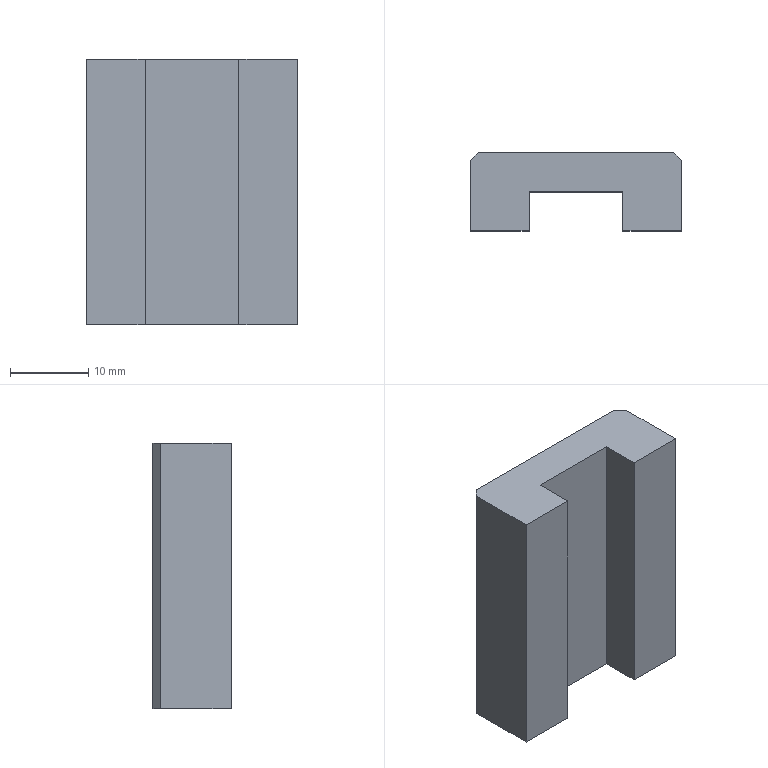Part | SolidWorks | features Chamfer 1, Extrusion 1, HoleWzd 1 | 1 solid | 28 faces | box 27 x 10 x 34 mm | volume 6954 mm3 | plane 12 | cylinder 8 | cone 8 | commonest cylinder face diameters 2.5 x8
STEP:
#1=CARTESIAN_POINT('',(-10.,-2.5,8.25));
#2=VERTEX_POINT('',#1);
#3=CARTESIAN_POINT('',(-10.,-2.5,10.75));
#4=VERTEX_POINT('',#3);
#5=CARTESIAN_POINT('',(-10.,-2.5,9.5));
#6=DIRECTION('',(0.,1.,0.));
#7=DIRECTION('',(0.,0.,1.));
#8=AXIS2_PLACEMENT_3D('',#5,#6,#7);
#9=CIRCLE('',#8,1.25);
#10=EDGE_CURVE('',#2,#4,#9,.T.);
#11=ORIENTED_EDGE('',*,*,#10,.F.);
#12=CARTESIAN_POINT('',(-10.,5.,8.25));
#13=VERTEX_POINT('',#12);
#14=CARTESIAN_POINT('',(-10.,5.,8.25));
#15=DIRECTION('',(0.,1.,0.));
#16=VECTOR('',#15,1000.);
#17=LINE('',#14,#16);
#18=EDGE_CURVE('',#2,#13,#17,.T.);
#19=ORIENTED_EDGE('',*,*,#18,.T.);
#20=CARTESIAN_POINT('',(-10.,5.,10.75));
#21=VERTEX_POINT('',#20);
#22=CARTESIAN_POINT('',(-10.,5.,9.5));
#23=DIRECTION('',(0.,1.,0.));
#24=DIRECTION('',(0.,0.,1.));
#25=AXIS2_PLACEMENT_3D('',#22,#23,#24);
#26=CIRCLE('',#25,1.25);
#27=EDGE_CURVE('',#13,#21,#26,.T.);
#28=ORIENTED_EDGE('',*,*,#27,.T.);
#29=CARTESIAN_POINT('',(-10.,5.,10.75));
#30=DIRECTION('',(0.,1.,0.));
#31=VECTOR('',#30,1000.);
#32=LINE('',#29,#31);
#33=EDGE_CURVE('',#4,#21,#32,.T.);
#34=ORIENTED_EDGE('',*,*,#33,.F.);
#35=EDGE_LOOP('',(#11,#19,#28,#34));
#36=FACE_OUTER_BOUND('',#35,.T.);
#37=CARTESIAN_POINT('',(-10.,5.,9.5));
#38=DIRECTION('',(0.,1.,0.));
#39=DIRECTION('',(0.,0.,1.));
#40=AXIS2_PLACEMENT_3D('',#37,#38,#39);
#41=CYLINDRICAL_SURFACE('',#40,1.25);
#42=ADVANCED_FACE('',(#36),#41,.F.);
#43=CARTESIAN_POINT('',(-10.,-3.251,9.5));
#44=VERTEX_POINT('',#43);
#45=CARTESIAN_POINT('',(-10.,-2.5,10.75));
#46=DIRECTION('',(0.,0.515,0.8572));
#47=VECTOR('',#46,1000.);
#48=LINE('',#45,#47);
#49=EDGE_CURVE('',#44,#4,#48,.T.);
#50=ORIENTED_EDGE('',*,*,#49,.F.);
#51=CARTESIAN_POINT('',(-10.,-2.5,8.25));
#52=DIRECTION('',(0.,0.515,-0.8572));
#53=VECTOR('',#52,1000.);
#54=LINE('',#51,#53);
#55=EDGE_CURVE('',#44,#2,#54,.T.);
#56=ORIENTED_EDGE('',*,*,#55,.T.);
#57=ORIENTED_EDGE('',*,*,#10,.T.);
#58=EDGE_LOOP('',(#50,#56,#57));
#59=FACE_OUTER_BOUND('',#58,.T.);
#60=CARTESIAN_POINT('',(-10.,-2.5,9.5));
#61=DIRECTION('',(0.,1.,0.));
#62=DIRECTION('',(0.,0.,1.));
#63=AXIS2_PLACEMENT_3D('',#60,#61,#62);
#64=CONICAL_SURFACE('',#63,1.25,1.03);
#65=ADVANCED_FACE('',(#59),#64,.F.);
#66=CARTESIAN_POINT('',(10.,-2.5,8.25));
#67=VERTEX_POINT('',#66);
#68=CARTESIAN_POINT('',(10.,-2.5,10.75));
#69=VERTEX_POINT('',#68);
#70=CARTESIAN_POINT('',(10.,-2.5,9.5));
#71=DIRECTION('',(0.,1.,0.));
#72=DIRECTION('',(0.,0.,1.));
#73=AXIS2_PLACEMENT_3D('',#70,#71,#72);
#74=CIRCLE('',#73,1.25);
#75=EDGE_CURVE('',#67,#69,#74,.T.);
#76=ORIENTED_EDGE('',*,*,#75,.F.);
#77=CARTESIAN_POINT('',(10.,5.,8.25));
#78=VERTEX_POINT('',#77);
#79=CARTESIAN_POINT('',(10.,5.,8.25));
#80=DIRECTION('',(0.,1.,0.));
#81=VECTOR('',#80,1000.);
#82=LINE('',#79,#81);
#83=EDGE_CURVE('',#67,#78,#82,.T.);
#84=ORIENTED_EDGE('',*,*,#83,.T.);
#85=CARTESIAN_POINT('',(10.,5.,10.75));
#86=VERTEX_POINT('',#85);
#87=CARTESIAN_POINT('',(10.,5.,9.5));
#88=DIRECTION('',(0.,1.,0.));
#89=DIRECTION('',(0.,0.,1.));
#90=AXIS2_PLACEMENT_3D('',#87,#88,#89);
#91=CIRCLE('',#90,1.25);
#92=EDGE_CURVE('',#78,#86,#91,.T.);
#93=ORIENTED_EDGE('',*,*,#92,.T.);
#94=CARTESIAN_POINT('',(10.,5.,10.75));
#95=DIRECTION('',(0.,1.,0.));
#96=VECTOR('',#95,1000.);
#97=LINE('',#94,#96);
#98=EDGE_CURVE('',#69,#86,#97,.T.);
#99=ORIENTED_EDGE('',*,*,#98,.F.);
#100=EDGE_LOOP('',(#76,#84,#93,#99));
#101=FACE_OUTER_BOUND('',#100,.T.);
#102=CARTESIAN_POINT('',(10.,5.,9.5));
#103=DIRECTION('',(0.,1.,0.));
#104=DIRECTION('',(0.,0.,1.));
#105=AXIS2_PLACEMENT_3D('',#102,#103,#104);
#106=CYLINDRICAL_SURFACE('',#105,1.25);
#107=ADVANCED_FACE('',(#101),#106,.F.);
#108=CARTESIAN_POINT('',(10.,-3.251,9.5));
#109=VERTEX_POINT('',#108);
#110=CARTESIAN_POINT('',(10.,-2.5,10.75));
#111=DIRECTION('',(0.,0.515,0.8572));
#112=VECTOR('',#111,1000.);
#113=LINE('',#110,#112);
#114=EDGE_CURVE('',#109,#69,#113,.T.);
#115=ORIENTED_EDGE('',*,*,#114,.F.);
#116=CARTESIAN_POINT('',(10.,-2.5,8.25));
#117=DIRECTION('',(0.,0.515,-0.8572));
#118=VECTOR('',#117,1000.);
#119=LINE('',#116,#118);
#120=EDGE_CURVE('',#109,#67,#119,.T.);
#121=ORIENTED_EDGE('',*,*,#120,.T.);
#122=ORIENTED_EDGE('',*,*,#75,.T.);
#123=EDGE_LOOP('',(#115,#121,#122));
#124=FACE_OUTER_BOUND('',#123,.T.);
#125=CARTESIAN_POINT('',(10.,-2.5,9.5));
#126=DIRECTION('',(0.,1.,0.));
#127=DIRECTION('',(0.,0.,1.));
#128=AXIS2_PLACEMENT_3D('',#125,#126,#127);
#129=CONICAL_SURFACE('',#128,1.25,1.03);
#130=ADVANCED_FACE('',(#124),#129,.F.);
#131=CARTESIAN_POINT('',(-10.,-2.5,23.25));
#132=VERTEX_POINT('',#131);
#133=CARTESIAN_POINT('',(-10.,-2.5,25.75));
#134=VERTEX_POINT('',#133);
#135=CARTESIAN_POINT('',(-10.,-2.5,24.5));
#136=DIRECTION('',(0.,1.,0.));
#137=DIRECTION('',(0.,0.,1.));
#138=AXIS2_PLACEMENT_3D('',#135,#136,#137);
#139=CIRCLE('',#138,1.25);
#140=EDGE_CURVE('',#132,#134,#139,.T.);
#141=ORIENTED_EDGE('',*,*,#140,.F.);
#142=CARTESIAN_POINT('',(-10.,5.,23.25));
#143=VERTEX_POINT('',#142);
#144=CARTESIAN_POINT('',(-10.,5.,23.25));
#145=DIRECTION('',(0.,1.,0.));
#146=VECTOR('',#145,1000.);
#147=LINE('',#144,#146);
#148=EDGE_CURVE('',#132,#143,#147,.T.);
#149=ORIENTED_EDGE('',*,*,#148,.T.);
#150=CARTESIAN_POINT('',(-10.,5.,25.75));
#151=VERTEX_POINT('',#150);
#152=CARTESIAN_POINT('',(-10.,5.,24.5));
#153=DIRECTION('',(0.,1.,0.));
#154=DIRECTION('',(0.,0.,1.));
#155=AXIS2_PLACEMENT_3D('',#152,#153,#154);
#156=CIRCLE('',#155,1.25);
#157=EDGE_CURVE('',#143,#151,#156,.T.);
#158=ORIENTED_EDGE('',*,*,#157,.T.);
#159=CARTESIAN_POINT('',(-10.,5.,25.75));
#160=DIRECTION('',(0.,1.,0.));
#161=VECTOR('',#160,1000.);
#162=LINE('',#159,#161);
#163=EDGE_CURVE('',#134,#151,#162,.T.);
#164=ORIENTED_EDGE('',*,*,#163,.F.);
#165=EDGE_LOOP('',(#141,#149,#158,#164));
#166=FACE_OUTER_BOUND('',#165,.T.);
#167=CARTESIAN_POINT('',(-10.,5.,24.5));
#168=DIRECTION('',(0.,1.,0.));
#169=DIRECTION('',(0.,0.,1.));
#170=AXIS2_PLACEMENT_3D('',#167,#168,#169);
#171=CYLINDRICAL_SURFACE('',#170,1.25);
#172=ADVANCED_FACE('',(#166),#171,.F.);
#173=CARTESIAN_POINT('',(-10.,-3.251,24.5));
#174=VERTEX_POINT('',#173);
#175=CARTESIAN_POINT('',(-10.,-2.5,25.75));
#176=DIRECTION('',(0.,0.515,0.8572));
#177=VECTOR('',#176,1000.);
#178=LINE('',#175,#177);
#179=EDGE_CURVE('',#174,#134,#178,.T.);
#180=ORIENTED_EDGE('',*,*,#179,.F.);
#181=CARTESIAN_POINT('',(-10.,-2.5,23.25));
#182=DIRECTION('',(0.,0.515,-0.8572));
#183=VECTOR('',#182,1000.);
#184=LINE('',#181,#183);
#185=EDGE_CURVE('',#174,#132,#184,.T.);
#186=ORIENTED_EDGE('',*,*,#185,.T.);
#187=ORIENTED_EDGE('',*,*,#140,.T.);
#188=EDGE_LOOP('',(#180,#186,#187));
#189=FACE_OUTER_BOUND('',#188,.T.);
#190=CARTESIAN_POINT('',(-10.,-2.5,24.5));
#191=DIRECTION('',(0.,1.,0.));
#192=DIRECTION('',(0.,0.,1.));
#193=AXIS2_PLACEMENT_3D('',#190,#191,#192);
#194=CONICAL_SURFACE('',#193,1.25,1.03);
#195=ADVANCED_FACE('',(#189),#194,.F.);
#196=CARTESIAN_POINT('',(10.,-2.5,23.25));
#197=VERTEX_POINT('',#196);
#198=CARTESIAN_POINT('',(10.,-2.5,25.75));
#199=VERTEX_POINT('',#198);
#200=CARTESIAN_POINT('',(10.,-2.5,24.5));
#201=DIRECTION('',(0.,1.,0.));
#202=DIRECTION('',(0.,0.,1.));
#203=AXIS2_PLACEMENT_3D('',#200,#201,#202);
#204=CIRCLE('',#203,1.25);
#205=EDGE_CURVE('',#197,#199,#204,.T.);
#206=ORIENTED_EDGE('',*,*,#205,.F.);
#207=CARTESIAN_POINT('',(10.,5.,23.25));
#208=VERTEX_POINT('',#207);
#209=CARTESIAN_POINT('',(10.,5.,23.25));
#210=DIRECTION('',(0.,1.,0.));
#211=VECTOR('',#210,1000.);
#212=LINE('',#209,#211);
#213=EDGE_CURVE('',#197,#208,#212,.T.);
#214=ORIENTED_EDGE('',*,*,#213,.T.);
#215=CARTESIAN_POINT('',(10.,5.,25.75));
#216=VERTEX_POINT('',#215);
#217=CARTESIAN_POINT('',(10.,5.,24.5));
#218=DIRECTION('',(0.,1.,0.));
#219=DIRECTION('',(0.,0.,1.));
#220=AXIS2_PLACEMENT_3D('',#217,#218,#219);
#221=CIRCLE('',#220,1.25);
#222=EDGE_CURVE('',#208,#216,#221,.T.);
#223=ORIENTED_EDGE('',*,*,#222,.T.);
#224=CARTESIAN_POINT('',(10.,5.,25.75));
#225=DIRECTION('',(0.,1.,0.));
#226=VECTOR('',#225,1000.);
#227=LINE('',#224,#226);
#228=EDGE_CURVE('',#199,#216,#227,.T.);
#229=ORIENTED_EDGE('',*,*,#228,.F.);
#230=EDGE_LOOP('',(#206,#214,#223,#229));
#231=FACE_OUTER_BOUND('',#230,.T.);
#232=CARTESIAN_POINT('',(10.,5.,24.5));
#233=DIRECTION('',(0.,1.,0.));
#234=DIRECTION('',(0.,0.,1.));
#235=AXIS2_PLACEMENT_3D('',#232,#233,#234);
#236=CYLINDRICAL_SURFACE('',#235,1.25);
#237=ADVANCED_FACE('',(#231),#236,.F.);
#238=CARTESIAN_POINT('',(10.,-3.251,24.5));
#239=VERTEX_POINT('',#238);
#240=CARTESIAN_POINT('',(10.,-2.5,25.75));
#241=DIRECTION('',(0.,0.515,0.8572));
#242=VECTOR('',#241,1000.);
#243=LINE('',#240,#242);
#244=EDGE_CURVE('',#239,#199,#243,.T.);
#245=ORIENTED_EDGE('',*,*,#244,.F.);
#246=CARTESIAN_POINT('',(10.,-2.5,23.25));
#247=DIRECTION('',(0.,0.515,-0.8572));
#248=VECTOR('',#247,1000.);
#249=LINE('',#246,#248);
#250=EDGE_CURVE('',#239,#197,#249,.T.);
#251=ORIENTED_EDGE('',*,*,#250,.T.);
#252=ORIENTED_EDGE('',*,*,#205,.T.);
#253=EDGE_LOOP('',(#245,#251,#252));
#254=FACE_OUTER_BOUND('',#253,.T.);
#255=CARTESIAN_POINT('',(10.,-2.5,24.5));
#256=DIRECTION('',(0.,1.,0.));
#257=DIRECTION('',(0.,0.,1.));
#258=AXIS2_PLACEMENT_3D('',#255,#256,#257);
#259=CONICAL_SURFACE('',#258,1.25,1.03);
#260=ADVANCED_FACE('',(#254),#259,.F.);
#261=CARTESIAN_POINT('',(-13.5,-5.,0.));
#262=VERTEX_POINT('',#261);
#263=CARTESIAN_POINT('',(-6.,-5.,0.));
#264=VERTEX_POINT('',#263);
#265=CARTESIAN_POINT('',(-6.,-5.,0.));
#266=DIRECTION('',(1.,0.,0.));
#267=VECTOR('',#266,1000.);
#268=LINE('',#265,#267);
#269=EDGE_CURVE('',#262,#264,#268,.T.);
#270=ORIENTED_EDGE('',*,*,#269,.T.);
#271=CARTESIAN_POINT('',(-6.,-5.,34.));
#272=VERTEX_POINT('',#271);
#273=CARTESIAN_POINT('',(-6.,-5.,34.));
#274=DIRECTION('',(0.,0.,-1.));
#275=VECTOR('',#274,1000.);
#276=LINE('',#273,#275);
#277=EDGE_CURVE('',#272,#264,#276,.T.);
#278=ORIENTED_EDGE('',*,*,#277,.F.);
#279=CARTESIAN_POINT('',(-13.5,-5.,34.));
#280=VERTEX_POINT('',#279);
#281=CARTESIAN_POINT('',(-6.,-5.,34.));
#282=DIRECTION('',(1.,0.,0.));
#283=VECTOR('',#282,1000.);
#284=LINE('',#281,#283);
#285=EDGE_CURVE('',#280,#272,#284,.T.);
#286=ORIENTED_EDGE('',*,*,#285,.F.);
#287=CARTESIAN_POINT('',(-13.5,-5.,34.));
#288=DIRECTION('',(0.,0.,-1.));
#289=VECTOR('',#288,1000.);
#290=LINE('',#287,#289);
#291=EDGE_CURVE('',#280,#262,#290,.T.);
#292=ORIENTED_EDGE('',*,*,#291,.T.);
#293=EDGE_LOOP('',(#270,#278,#286,#292));
#294=FACE_OUTER_BOUND('',#293,.T.);
#295=CARTESIAN_POINT('',(-6.,-5.,34.));
#296=DIRECTION('',(0.,1.,0.));
#297=DIRECTION('',(-1.,0.,0.));
#298=AXIS2_PLACEMENT_3D('',#295,#296,#297);
#299=PLANE('',#298);
#300=ADVANCED_FACE('',(#294),#299,.F.);
#301=CARTESIAN_POINT('',(-6.,0.,0.));
#302=VERTEX_POINT('',#301);
#303=CARTESIAN_POINT('',(-6.,0.,0.));
#304=DIRECTION('',(0.,1.,0.));
#305=VECTOR('',#304,1000.);
#306=LINE('',#303,#305);
#307=EDGE_CURVE('',#264,#302,#306,.T.);
#308=ORIENTED_EDGE('',*,*,#307,.T.);
#309=CARTESIAN_POINT('',(-6.,0.,34.));
#310=VERTEX_POINT('',#309);
#311=CARTESIAN_POINT('',(-6.,0.,34.));
#312=DIRECTION('',(0.,0.,-1.));
#313=VECTOR('',#312,1000.);
#314=LINE('',#311,#313);
#315=EDGE_CURVE('',#310,#302,#314,.T.);
#316=ORIENTED_EDGE('',*,*,#315,.F.);
#317=CARTESIAN_POINT('',(-6.,0.,34.));
#318=DIRECTION('',(0.,1.,0.));
#319=VECTOR('',#318,1000.);
#320=LINE('',#317,#319);
#321=EDGE_CURVE('',#272,#310,#320,.T.);
#322=ORIENTED_EDGE('',*,*,#321,.F.);
#323=ORIENTED_EDGE('',*,*,#277,.T.);
#324=EDGE_LOOP('',(#308,#316,#322,#323));
#325=FACE_OUTER_BOUND('',#324,.T.);
#326=CARTESIAN_POINT('',(-6.,0.,34.));
#327=DIRECTION('',(-1.,0.,0.));
#328=DIRECTION('',(0.,0.,1.));
#329=AXIS2_PLACEMENT_3D('',#326,#327,#328);
#330=PLANE('',#329);
#331=ADVANCED_FACE('',(#325),#330,.F.);
#332=CARTESIAN_POINT('',(6.,0.,0.));
#333=VERTEX_POINT('',#332);
#334=CARTESIAN_POINT('',(-6.,0.,0.));
#335=DIRECTION('',(1.,0.,0.));
#336=VECTOR('',#335,1000.);
#337=LINE('',#334,#336);
#338=EDGE_CURVE('',#302,#333,#337,.T.);
#339=ORIENTED_EDGE('',*,*,#338,.T.);
#340=CARTESIAN_POINT('',(6.,0.,34.));
#341=VERTEX_POINT('',#340);
#342=CARTESIAN_POINT('',(6.,0.,34.));
#343=DIRECTION('',(0.,0.,-1.));
#344=VECTOR('',#343,1000.);
#345=LINE('',#342,#344);
#346=EDGE_CURVE('',#341,#333,#345,.T.);
#347=ORIENTED_EDGE('',*,*,#346,.F.);
#348=CARTESIAN_POINT('',(-6.,0.,34.));
#349=DIRECTION('',(1.,0.,0.));
#350=VECTOR('',#349,1000.);
#351=LINE('',#348,#350);
#352=EDGE_CURVE('',#310,#341,#351,.T.);
#353=ORIENTED_EDGE('',*,*,#352,.F.);
#354=ORIENTED_EDGE('',*,*,#315,.T.);
#355=EDGE_LOOP('',(#339,#347,#353,#354));
#356=FACE_OUTER_BOUND('',#355,.T.);
#357=CARTESIAN_POINT('',(-6.,0.,34.));
#358=DIRECTION('',(0.,1.,0.));
#359=DIRECTION('',(0.,0.,1.));
#360=AXIS2_PLACEMENT_3D('',#357,#358,#359);
#361=PLANE('',#360);
#362=ADVANCED_FACE('',(#356),#361,.F.);
#363=CARTESIAN_POINT('',(6.,-5.,0.));
#364=VERTEX_POINT('',#363);
#365=CARTESIAN_POINT('',(6.,0.,0.));
#366=DIRECTION('',(0.,-1.,0.));
#367=VECTOR('',#366,1000.);
#368=LINE('',#365,#367);
#369=EDGE_CURVE('',#333,#364,#368,.T.);
#370=ORIENTED_EDGE('',*,*,#369,.T.);
#371=CARTESIAN_POINT('',(6.,-5.,34.));
#372=VERTEX_POINT('',#371);
#373=CARTESIAN_POINT('',(6.,-5.,34.));
#374=DIRECTION('',(0.,0.,-1.));
#375=VECTOR('',#374,1000.);
#376=LINE('',#373,#375);
#377=EDGE_CURVE('',#372,#364,#376,.T.);
#378=ORIENTED_EDGE('',*,*,#377,.F.);
#379=CARTESIAN_POINT('',(6.,0.,34.));
#380=DIRECTION('',(0.,-1.,0.));
#381=VECTOR('',#380,1000.);
#382=LINE('',#379,#381);
#383=EDGE_CURVE('',#341,#372,#382,.T.);
#384=ORIENTED_EDGE('',*,*,#383,.F.);
#385=ORIENTED_EDGE('',*,*,#346,.T.);
#386=EDGE_LOOP('',(#370,#378,#384,#385));
#387=FACE_OUTER_BOUND('',#386,.T.);
#388=CARTESIAN_POINT('',(6.,0.,34.));
#389=DIRECTION('',(1.,0.,0.));
#390=DIRECTION('',(0.,0.,-1.));
#391=AXIS2_PLACEMENT_3D('',#388,#389,#390);
#392=PLANE('',#391);
#393=ADVANCED_FACE('',(#387),#392,.F.);
#394=CARTESIAN_POINT('',(13.5,-5.,0.));
#395=VERTEX_POINT('',#394);
#396=CARTESIAN_POINT('',(13.5,-5.,0.));
#397=DIRECTION('',(1.,0.,0.));
#398=VECTOR('',#397,1000.);
#399=LINE('',#396,#398);
#400=EDGE_CURVE('',#364,#395,#399,.T.);
#401=ORIENTED_EDGE('',*,*,#400,.T.);
#402=CARTESIAN_POINT('',(13.5,-5.,34.));
#403=VERTEX_POINT('',#402);
#404=CARTESIAN_POINT('',(13.5,-5.,34.));
#405=DIRECTION('',(0.,0.,-1.));
#406=VECTOR('',#405,1000.);
#407=LINE('',#404,#406);
#408=EDGE_CURVE('',#403,#395,#407,.T.);
#409=ORIENTED_EDGE('',*,*,#408,.F.);
#410=CARTESIAN_POINT('',(13.5,-5.,34.));
#411=DIRECTION('',(1.,0.,0.));
#412=VECTOR('',#411,1000.);
#413=LINE('',#410,#412);
#414=EDGE_CURVE('',#372,#403,#413,.T.);
#415=ORIENTED_EDGE('',*,*,#414,.F.);
#416=ORIENTED_EDGE('',*,*,#377,.T.);
#417=EDGE_LOOP('',(#401,#409,#415,#416));
#418=FACE_OUTER_BOUND('',#417,.T.);
#419=CARTESIAN_POINT('',(13.5,-5.,34.));
#420=DIRECTION('',(0.,1.,0.));
#421=DIRECTION('',(-1.,0.,0.));
#422=AXIS2_PLACEMENT_3D('',#419,#420,#421);
#423=PLANE('',#422);
#424=ADVANCED_FACE('',(#418),#423,.F.);
#425=CARTESIAN_POINT('',(13.5,4.,0.));
#426=VERTEX_POINT('',#425);
#427=CARTESIAN_POINT('',(13.5,5.,0.));
#428=DIRECTION('',(0.,1.,0.));
#429=VECTOR('',#428,1000.);
#430=LINE('',#427,#429);
#431=EDGE_CURVE('',#395,#426,#430,.T.);
#432=ORIENTED_EDGE('',*,*,#431,.T.);
#433=CARTESIAN_POINT('',(13.5,4.,34.));
#434=VERTEX_POINT('',#433);
#435=CARTESIAN_POINT('',(13.5,4.,34.));
#436=DIRECTION('',(0.,0.,1.));
#437=VECTOR('',#436,1000.);
#438=LINE('',#435,#437);
#439=EDGE_CURVE('',#426,#434,#438,.T.);
#440=ORIENTED_EDGE('',*,*,#439,.T.);
#441=CARTESIAN_POINT('',(13.5,5.,34.));
#442=DIRECTION('',(0.,1.,0.));
#443=VECTOR('',#442,1000.);
#444=LINE('',#441,#443);
#445=EDGE_CURVE('',#403,#434,#444,.T.);
#446=ORIENTED_EDGE('',*,*,#445,.F.);
#447=ORIENTED_EDGE('',*,*,#408,.T.);
#448=EDGE_LOOP('',(#432,#440,#446,#447));
#449=FACE_OUTER_BOUND('',#448,.T.);
#450=CARTESIAN_POINT('',(13.5,5.,34.));
#451=DIRECTION('',(-1.,0.,0.));
#452=DIRECTION('',(0.,-1.,0.));
#453=AXIS2_PLACEMENT_3D('',#450,#451,#452);
#454=PLANE('',#453);
#455=ADVANCED_FACE('',(#449),#454,.F.);
#456=CARTESIAN_POINT('',(-10.,5.,9.5));
#457=DIRECTION('',(0.,1.,0.));
#458=DIRECTION('',(0.,0.,1.));
#459=AXIS2_PLACEMENT_3D('',#456,#457,#458);
#460=CIRCLE('',#459,1.25);
#461=EDGE_CURVE('',#21,#13,#460,.T.);
#462=ORIENTED_EDGE('',*,*,#461,.F.);
#463=ORIENTED_EDGE('',*,*,#27,.F.);
#464=EDGE_LOOP('',(#462,#463));
#465=FACE_BOUND('',#464,.T.);
#466=CARTESIAN_POINT('',(10.,5.,9.5));
#467=DIRECTION('',(0.,1.,0.));
#468=DIRECTION('',(0.,0.,1.));
#469=AXIS2_PLACEMENT_3D('',#466,#467,#468);
#470=CIRCLE('',#469,1.25);
#471=EDGE_CURVE('',#86,#78,#470,.T.);
#472=ORIENTED_EDGE('',*,*,#471,.F.);
#473=ORIENTED_EDGE('',*,*,#92,.F.);
#474=EDGE_LOOP('',(#472,#473));
#475=FACE_BOUND('',#474,.T.);
#476=CARTESIAN_POINT('',(-10.,5.,24.5));
#477=DIRECTION('',(0.,1.,0.));
#478=DIRECTION('',(0.,0.,1.));
#479=AXIS2_PLACEMENT_3D('',#476,#477,#478);
#480=CIRCLE('',#479,1.25);
#481=EDGE_CURVE('',#151,#143,#480,.T.);
#482=ORIENTED_EDGE('',*,*,#481,.F.);
#483=ORIENTED_EDGE('',*,*,#157,.F.);
#484=EDGE_LOOP('',(#482,#483));
#485=FACE_BOUND('',#484,.T.);
#486=CARTESIAN_POINT('',(10.,5.,24.5));
#487=DIRECTION('',(0.,1.,0.));
#488=DIRECTION('',(0.,0.,1.));
#489=AXIS2_PLACEMENT_3D('',#486,#487,#488);
#490=CIRCLE('',#489,1.25);
#491=EDGE_CURVE('',#216,#208,#490,.T.);
#492=ORIENTED_EDGE('',*,*,#491,.F.);
#493=ORIENTED_EDGE('',*,*,#222,.F.);
#494=EDGE_LOOP('',(#492,#493));
#495=FACE_BOUND('',#494,.T.);
#496=CARTESIAN_POINT('',(12.5,5.,34.));
#497=VERTEX_POINT('',#496);
#498=CARTESIAN_POINT('',(-12.5,5.,34.));
#499=VERTEX_POINT('',#498);
#500=CARTESIAN_POINT('',(13.5,5.,34.));
#501=DIRECTION('',(-1.,0.,0.));
#502=VECTOR('',#501,1000.);
#503=LINE('',#500,#502);
#504=EDGE_CURVE('',#497,#499,#503,.T.);
#505=ORIENTED_EDGE('',*,*,#504,.F.);
#506=CARTESIAN_POINT('',(12.5,5.,0.));
#507=VERTEX_POINT('',#506);
#508=CARTESIAN_POINT('',(12.5,5.,34.));
#509=DIRECTION('',(0.,0.,-1.));
#510=VECTOR('',#509,1000.);
#511=LINE('',#508,#510);
#512=EDGE_CURVE('',#497,#507,#511,.T.);
#513=ORIENTED_EDGE('',*,*,#512,.T.);
#514=CARTESIAN_POINT('',(-12.5,5.,0.));
#515=VERTEX_POINT('',#514);
#516=CARTESIAN_POINT('',(13.5,5.,0.));
#517=DIRECTION('',(-1.,0.,0.));
#518=VECTOR('',#517,1000.);
#519=LINE('',#516,#518);
#520=EDGE_CURVE('',#507,#515,#519,.T.);
#521=ORIENTED_EDGE('',*,*,#520,.T.);
#522=CARTESIAN_POINT('',(-12.5,5.,34.));
#523=DIRECTION('',(0.,0.,1.));
#524=VECTOR('',#523,1000.);
#525=LINE('',#522,#524);
#526=EDGE_CURVE('',#515,#499,#525,.T.);
#527=ORIENTED_EDGE('',*,*,#526,.T.);
#528=EDGE_LOOP('',(#505,#513,#521,#527));
#529=FACE_OUTER_BOUND('',#528,.T.);
#530=CARTESIAN_POINT('',(13.5,5.,34.));
#531=DIRECTION('',(0.,-1.,0.));
#532=DIRECTION('',(1.,0.,0.));
#533=AXIS2_PLACEMENT_3D('',#530,#531,#532);
#534=PLANE('',#533);
#535=ADVANCED_FACE('',(#465,#475,#485,#495,#529),#534,.F.);
#536=CARTESIAN_POINT('',(-13.5,4.,34.));
#537=VERTEX_POINT('',#536);
#538=CARTESIAN_POINT('',(-13.5,5.,34.));
#539=DIRECTION('',(0.,-1.,0.));
#540=VECTOR('',#539,1000.);
#541=LINE('',#538,#540);
#542=EDGE_CURVE('',#537,#280,#541,.T.);
#543=ORIENTED_EDGE('',*,*,#542,.F.);
#544=CARTESIAN_POINT('',(-13.5,4.,0.));
#545=VERTEX_POINT('',#544);
#546=CARTESIAN_POINT('',(-13.5,4.,34.));
#547=DIRECTION('',(0.,0.,-1.));
#548=VECTOR('',#547,1000.);
#549=LINE('',#546,#548);
#550=EDGE_CURVE('',#537,#545,#549,.T.);
#551=ORIENTED_EDGE('',*,*,#550,.T.);
#552=CARTESIAN_POINT('',(-13.5,5.,0.));
#553=DIRECTION('',(0.,-1.,0.));
#554=VECTOR('',#553,1000.);
#555=LINE('',#552,#554);
#556=EDGE_CURVE('',#545,#262,#555,.T.);
#557=ORIENTED_EDGE('',*,*,#556,.T.);
#558=ORIENTED_EDGE('',*,*,#291,.F.);
#559=EDGE_LOOP('',(#543,#551,#557,#558));
#560=FACE_OUTER_BOUND('',#559,.T.);
#561=CARTESIAN_POINT('',(-13.5,5.,34.));
#562=DIRECTION('',(1.,0.,0.));
#563=DIRECTION('',(0.,1.,0.));
#564=AXIS2_PLACEMENT_3D('',#561,#562,#563);
#565=PLANE('',#564);
#566=ADVANCED_FACE('',(#560),#565,.F.);
#567=ORIENTED_EDGE('',*,*,#445,.T.);
#568=CARTESIAN_POINT('',(8.75,8.75,34.));
#569=DIRECTION('',(-0.7071,0.7071,0.));
#570=VECTOR('',#569,1000.);
#571=LINE('',#568,#570);
#572=EDGE_CURVE('',#434,#497,#571,.T.);
#573=ORIENTED_EDGE('',*,*,#572,.T.);
#574=ORIENTED_EDGE('',*,*,#504,.T.);
#575=CARTESIAN_POINT('',(-8.75,8.75,34.));
#576=DIRECTION('',(-0.7071,-0.7071,0.));
#577=VECTOR('',#576,1000.);
#578=LINE('',#575,#577);
#579=EDGE_CURVE('',#499,#537,#578,.T.);
#580=ORIENTED_EDGE('',*,*,#579,.T.);
#581=ORIENTED_EDGE('',*,*,#542,.T.);
#582=ORIENTED_EDGE('',*,*,#285,.T.);
#583=ORIENTED_EDGE('',*,*,#321,.T.);
#584=ORIENTED_EDGE('',*,*,#352,.T.);
#585=ORIENTED_EDGE('',*,*,#383,.T.);
#586=ORIENTED_EDGE('',*,*,#414,.T.);
#587=EDGE_LOOP('',(#567,#573,#574,#580,#581,#582,#583,#584,#585,#586));
#588=FACE_OUTER_BOUND('',#587,.T.);
#589=CARTESIAN_POINT('',(0.,0.,34.));
#590=DIRECTION('',(0.,0.,1.));
#591=DIRECTION('',(1.,0.,0.));
#592=AXIS2_PLACEMENT_3D('',#589,#590,#591);
#593=PLANE('',#592);
#594=ADVANCED_FACE('',(#588),#593,.T.);
#595=ORIENTED_EDGE('',*,*,#520,.F.);
#596=CARTESIAN_POINT('',(12.5,5.,0.));
#597=DIRECTION('',(0.7071,-0.7071,0.));
#598=VECTOR('',#597,1000.);
#599=LINE('',#596,#598);
#600=EDGE_CURVE('',#507,#426,#599,.T.);
#601=ORIENTED_EDGE('',*,*,#600,.T.);
#602=ORIENTED_EDGE('',*,*,#431,.F.);
#603=ORIENTED_EDGE('',*,*,#400,.F.);
#604=ORIENTED_EDGE('',*,*,#369,.F.);
#605=ORIENTED_EDGE('',*,*,#338,.F.);
#606=ORIENTED_EDGE('',*,*,#307,.F.);
#607=ORIENTED_EDGE('',*,*,#269,.F.);
#608=ORIENTED_EDGE('',*,*,#556,.F.);
#609=CARTESIAN_POINT('',(-13.5,4.,0.));
#610=DIRECTION('',(0.7071,0.7071,0.));
#611=VECTOR('',#610,1000.);
#612=LINE('',#609,#611);
#613=EDGE_CURVE('',#545,#515,#612,.T.);
#614=ORIENTED_EDGE('',*,*,#613,.T.);
#615=EDGE_LOOP('',(#595,#601,#602,#603,#604,#605,#606,#607,#608,#614));
#616=FACE_OUTER_BOUND('',#615,.T.);
#617=CARTESIAN_POINT('',(0.,0.,0.));
#618=DIRECTION('',(0.,0.,1.));
#619=DIRECTION('',(1.,0.,0.));
#620=AXIS2_PLACEMENT_3D('',#617,#618,#619);
#621=PLANE('',#620);
#622=ADVANCED_FACE('',(#616),#621,.F.);
#623=ORIENTED_EDGE('',*,*,#250,.F.);
#624=ORIENTED_EDGE('',*,*,#244,.T.);
#625=CARTESIAN_POINT('',(10.,-2.5,24.5));
#626=DIRECTION('',(0.,1.,0.));
#627=DIRECTION('',(0.,0.,1.));
#628=AXIS2_PLACEMENT_3D('',#625,#626,#627);
#629=CIRCLE('',#628,1.25);
#630=EDGE_CURVE('',#199,#197,#629,.T.);
#631=ORIENTED_EDGE('',*,*,#630,.T.);
#632=EDGE_LOOP('',(#623,#624,#631));
#633=FACE_OUTER_BOUND('',#632,.T.);
#634=CARTESIAN_POINT('',(10.,-2.5,24.5));
#635=DIRECTION('',(0.,1.,0.));
#636=DIRECTION('',(0.,0.,1.));
#637=AXIS2_PLACEMENT_3D('',#634,#635,#636);
#638=CONICAL_SURFACE('',#637,1.25,1.03);
#639=ADVANCED_FACE('',(#633),#638,.F.);
#640=ORIENTED_EDGE('',*,*,#213,.F.);
#641=ORIENTED_EDGE('',*,*,#630,.F.);
#642=ORIENTED_EDGE('',*,*,#228,.T.);
#643=ORIENTED_EDGE('',*,*,#491,.T.);
#644=EDGE_LOOP('',(#640,#641,#642,#643));
#645=FACE_OUTER_BOUND('',#644,.T.);
#646=CARTESIAN_POINT('',(10.,5.,24.5));
#647=DIRECTION('',(0.,1.,0.));
#648=DIRECTION('',(0.,0.,1.));
#649=AXIS2_PLACEMENT_3D('',#646,#647,#648);
#650=CYLINDRICAL_SURFACE('',#649,1.25);
#651=ADVANCED_FACE('',(#645),#650,.F.);
#652=ORIENTED_EDGE('',*,*,#185,.F.);
#653=ORIENTED_EDGE('',*,*,#179,.T.);
#654=CARTESIAN_POINT('',(-10.,-2.5,24.5));
#655=DIRECTION('',(0.,1.,0.));
#656=DIRECTION('',(0.,0.,1.));
#657=AXIS2_PLACEMENT_3D('',#654,#655,#656);
#658=CIRCLE('',#657,1.25);
#659=EDGE_CURVE('',#134,#132,#658,.T.);
#660=ORIENTED_EDGE('',*,*,#659,.T.);
#661=EDGE_LOOP('',(#652,#653,#660));
#662=FACE_OUTER_BOUND('',#661,.T.);
#663=CARTESIAN_POINT('',(-10.,-2.5,24.5));
#664=DIRECTION('',(0.,1.,0.));
#665=DIRECTION('',(0.,0.,1.));
#666=AXIS2_PLACEMENT_3D('',#663,#664,#665);
#667=CONICAL_SURFACE('',#666,1.25,1.03);
#668=ADVANCED_FACE('',(#662),#667,.F.);
#669=ORIENTED_EDGE('',*,*,#148,.F.);
#670=ORIENTED_EDGE('',*,*,#659,.F.);
#671=ORIENTED_EDGE('',*,*,#163,.T.);
#672=ORIENTED_EDGE('',*,*,#481,.T.);
#673=EDGE_LOOP('',(#669,#670,#671,#672));
#674=FACE_OUTER_BOUND('',#673,.T.);
#675=CARTESIAN_POINT('',(-10.,5.,24.5));
#676=DIRECTION('',(0.,1.,0.));
#677=DIRECTION('',(0.,0.,1.));
#678=AXIS2_PLACEMENT_3D('',#675,#676,#677);
#679=CYLINDRICAL_SURFACE('',#678,1.25);
#680=ADVANCED_FACE('',(#674),#679,.F.);
#681=ORIENTED_EDGE('',*,*,#120,.F.);
#682=ORIENTED_EDGE('',*,*,#114,.T.);
#683=CARTESIAN_POINT('',(10.,-2.5,9.5));
#684=DIRECTION('',(0.,1.,0.));
#685=DIRECTION('',(0.,0.,1.));
#686=AXIS2_PLACEMENT_3D('',#683,#684,#685);
#687=CIRCLE('',#686,1.25);
#688=EDGE_CURVE('',#69,#67,#687,.T.);
#689=ORIENTED_EDGE('',*,*,#688,.T.);
#690=EDGE_LOOP('',(#681,#682,#689));
#691=FACE_OUTER_BOUND('',#690,.T.);
#692=CARTESIAN_POINT('',(10.,-2.5,9.5));
#693=DIRECTION('',(0.,1.,0.));
#694=DIRECTION('',(0.,0.,1.));
#695=AXIS2_PLACEMENT_3D('',#692,#693,#694);
#696=CONICAL_SURFACE('',#695,1.25,1.03);
#697=ADVANCED_FACE('',(#691),#696,.F.);
#698=ORIENTED_EDGE('',*,*,#83,.F.);
#699=ORIENTED_EDGE('',*,*,#688,.F.);
#700=ORIENTED_EDGE('',*,*,#98,.T.);
#701=ORIENTED_EDGE('',*,*,#471,.T.);
#702=EDGE_LOOP('',(#698,#699,#700,#701));
#703=FACE_OUTER_BOUND('',#702,.T.);
#704=CARTESIAN_POINT('',(10.,5.,9.5));
#705=DIRECTION('',(0.,1.,0.));
#706=DIRECTION('',(0.,0.,1.));
#707=AXIS2_PLACEMENT_3D('',#704,#705,#706);
#708=CYLINDRICAL_SURFACE('',#707,1.25);
#709=ADVANCED_FACE('',(#703),#708,.F.);
#710=ORIENTED_EDGE('',*,*,#55,.F.);
#711=ORIENTED_EDGE('',*,*,#49,.T.);
#712=CARTESIAN_POINT('',(-10.,-2.5,9.5));
#713=DIRECTION('',(0.,1.,0.));
#714=DIRECTION('',(0.,0.,1.));
#715=AXIS2_PLACEMENT_3D('',#712,#713,#714);
#716=CIRCLE('',#715,1.25);
#717=EDGE_CURVE('',#4,#2,#716,.T.);
#718=ORIENTED_EDGE('',*,*,#717,.T.);
#719=EDGE_LOOP('',(#710,#711,#718));
#720=FACE_OUTER_BOUND('',#719,.T.);
#721=CARTESIAN_POINT('',(-10.,-2.5,9.5));
#722=DIRECTION('',(0.,1.,0.));
#723=DIRECTION('',(0.,0.,1.));
#724=AXIS2_PLACEMENT_3D('',#721,#722,#723);
#725=CONICAL_SURFACE('',#724,1.25,1.03);
#726=ADVANCED_FACE('',(#720),#725,.F.);
#727=ORIENTED_EDGE('',*,*,#18,.F.);
#728=ORIENTED_EDGE('',*,*,#717,.F.);
#729=ORIENTED_EDGE('',*,*,#33,.T.);
#730=ORIENTED_EDGE('',*,*,#461,.T.);
#731=EDGE_LOOP('',(#727,#728,#729,#730));
#732=FACE_OUTER_BOUND('',#731,.T.);
#733=CARTESIAN_POINT('',(-10.,5.,9.5));
#734=DIRECTION('',(0.,1.,0.));
#735=DIRECTION('',(0.,0.,1.));
#736=AXIS2_PLACEMENT_3D('',#733,#734,#735);
#737=CYLINDRICAL_SURFACE('',#736,1.25);
#738=ADVANCED_FACE('',(#732),#737,.F.);
#739=ORIENTED_EDGE('',*,*,#572,.F.);
#740=ORIENTED_EDGE('',*,*,#439,.F.);
#741=ORIENTED_EDGE('',*,*,#600,.F.);
#742=ORIENTED_EDGE('',*,*,#512,.F.);
#743=EDGE_LOOP('',(#739,#740,#741,#742));
#744=FACE_OUTER_BOUND('',#743,.T.);
#745=CARTESIAN_POINT('',(12.5,5.,34.));
#746=DIRECTION('',(-0.7071,-0.7071,0.));
#747=DIRECTION('',(0.,0.,-1.));
#748=AXIS2_PLACEMENT_3D('',#745,#746,#747);
#749=PLANE('',#748);
#750=ADVANCED_FACE('',(#744),#749,.F.);
#751=ORIENTED_EDGE('',*,*,#579,.F.);
#752=ORIENTED_EDGE('',*,*,#526,.F.);
#753=ORIENTED_EDGE('',*,*,#613,.F.);
#754=ORIENTED_EDGE('',*,*,#550,.F.);
#755=EDGE_LOOP('',(#751,#752,#753,#754));
#756=FACE_OUTER_BOUND('',#755,.T.);
#757=CARTESIAN_POINT('',(-13.5,4.,34.));
#758=DIRECTION('',(0.7071,-0.7071,0.));
#759=DIRECTION('',(0.,0.,-1.));
#760=AXIS2_PLACEMENT_3D('',#757,#758,#759);
#761=PLANE('',#760);
#762=ADVANCED_FACE('',(#756),#761,.F.);
#763=CLOSED_SHELL('',(#42,#65,#107,#130,#172,#195,#237,#260,#300,#331,#362,#393,#424,#455,#535,#566,#594,#622,#639,#651,#668,#680,#697,#709,#726,#738,#750,#762));
#764=MANIFOLD_SOLID_BREP('',#763);
#765=CARTESIAN_POINT('',(0.,0.,0.));
#766=DIRECTION('',(0.,0.,1.));
#767=DIRECTION('',(1.,0.,0.));
#768=AXIS2_PLACEMENT_3D('',#765,#766,#767);
#769=(LENGTH_UNIT()NAMED_UNIT(*)SI_UNIT(.MILLI.,.METRE.));
#770=UNCERTAINTY_MEASURE_WITH_UNIT(LENGTH_MEASURE(0.00001),#769,'','');
#771=(NAMED_UNIT(*)PLANE_ANGLE_UNIT()SI_UNIT($,.RADIAN.));
#772=(NAMED_UNIT(*)SI_UNIT($,.STERADIAN.)SOLID_ANGLE_UNIT());
#773=(GEOMETRIC_REPRESENTATION_CONTEXT(3)GLOBAL_UNCERTAINTY_ASSIGNED_CONTEXT((#770))GLOBAL_UNIT_ASSIGNED_CONTEXT((#769,#771,#772))REPRESENTATION_CONTEXT('',''));
#774=ADVANCED_BREP_SHAPE_REPRESENTATION('',(#764,#768),#773);